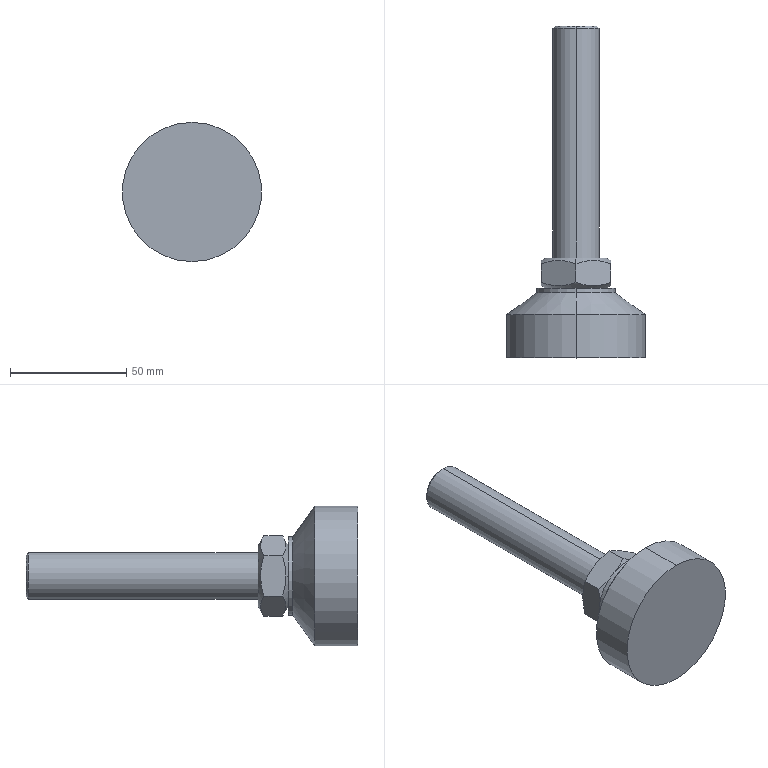Part | SolidWorks | features BaseBody 1 | 1 solid | 24 faces | box 60 x 143 x 60 mm | volume 112312 mm3 | plane 10 | cone 8 | cylinder 6 | commonest cylinder face diameters 20 x2 34 x2 60 x2
STEP:
#1=CARTESIAN_POINT('',(0.,43.,10.));
#2=VERTEX_POINT('',#1);
#3=CARTESIAN_POINT('',(0.,43.,-10.));
#4=VERTEX_POINT('',#3);
#5=CARTESIAN_POINT('',(0.,43.,0.));
#6=DIRECTION('',(0.,1.,0.));
#7=DIRECTION('',(0.,0.,1.));
#8=AXIS2_PLACEMENT_3D('',#5,#6,#7);
#9=CIRCLE('',#8,10.);
#10=EDGE_CURVE('',#2,#4,#9,.T.);
#11=ORIENTED_EDGE('',*,*,#10,.T.);
#12=CARTESIAN_POINT('',(0.,142.,-10.));
#13=VERTEX_POINT('',#12);
#14=CARTESIAN_POINT('',(0.,500.,-10.));
#15=DIRECTION('',(0.,1.,0.));
#16=VECTOR('',#15,1000.);
#17=LINE('',#14,#16);
#18=EDGE_CURVE('',#4,#13,#17,.T.);
#19=ORIENTED_EDGE('',*,*,#18,.T.);
#20=CARTESIAN_POINT('',(0.,142.,10.));
#21=VERTEX_POINT('',#20);
#22=CARTESIAN_POINT('',(0.,142.,0.));
#23=DIRECTION('',(0.,-1.,0.));
#24=DIRECTION('',(0.,0.,1.));
#25=AXIS2_PLACEMENT_3D('',#22,#23,#24);
#26=CIRCLE('',#25,10.);
#27=EDGE_CURVE('',#13,#21,#26,.T.);
#28=ORIENTED_EDGE('',*,*,#27,.T.);
#29=CARTESIAN_POINT('',(0.,500.,10.));
#30=DIRECTION('',(0.,1.,0.));
#31=VECTOR('',#30,1000.);
#32=LINE('',#29,#31);
#33=EDGE_CURVE('',#2,#21,#32,.T.);
#34=ORIENTED_EDGE('',*,*,#33,.F.);
#35=EDGE_LOOP('',(#11,#19,#28,#34));
#36=FACE_OUTER_BOUND('',#35,.T.);
#37=CARTESIAN_POINT('',(0.,500.,0.));
#38=DIRECTION('',(0.,1.,0.));
#39=DIRECTION('',(0.,0.,1.));
#40=AXIS2_PLACEMENT_3D('',#37,#38,#39);
#41=CYLINDRICAL_SURFACE('',#40,10.);
#42=ADVANCED_FACE('',(#36),#41,.T.);
#43=CARTESIAN_POINT('',(0.,143.,-9.));
#44=VERTEX_POINT('',#43);
#45=CARTESIAN_POINT('',(0.,143.,9.));
#46=VERTEX_POINT('',#45);
#47=CARTESIAN_POINT('',(0.,143.,0.));
#48=DIRECTION('',(0.,-1.,0.));
#49=DIRECTION('',(0.,0.,-1.));
#50=AXIS2_PLACEMENT_3D('',#47,#48,#49);
#51=CIRCLE('',#50,9.);
#52=EDGE_CURVE('',#44,#46,#51,.T.);
#53=ORIENTED_EDGE('',*,*,#52,.T.);
#54=CARTESIAN_POINT('',(0.,142.,10.));
#55=DIRECTION('',(0.,-0.7071,0.7071));
#56=VECTOR('',#55,1000.);
#57=LINE('',#54,#56);
#58=EDGE_CURVE('',#46,#21,#57,.T.);
#59=ORIENTED_EDGE('',*,*,#58,.T.);
#60=ORIENTED_EDGE('',*,*,#27,.F.);
#61=CARTESIAN_POINT('',(0.,142.,-10.));
#62=DIRECTION('',(0.,-0.7071,-0.7071));
#63=VECTOR('',#62,1000.);
#64=LINE('',#61,#63);
#65=EDGE_CURVE('',#44,#13,#64,.T.);
#66=ORIENTED_EDGE('',*,*,#65,.F.);
#67=EDGE_LOOP('',(#53,#59,#60,#66));
#68=FACE_OUTER_BOUND('',#67,.T.);
#69=CARTESIAN_POINT('',(0.,142.,0.));
#70=DIRECTION('',(0.,-1.,0.));
#71=DIRECTION('',(0.,0.,-1.));
#72=AXIS2_PLACEMENT_3D('',#69,#70,#71);
#73=CONICAL_SURFACE('',#72,10.,0.7854);
#74=ADVANCED_FACE('',(#68),#73,.T.);
#75=CARTESIAN_POINT('',(0.,43.,-13.1));
#76=VERTEX_POINT('',#75);
#77=CARTESIAN_POINT('',(0.,43.,13.1));
#78=VERTEX_POINT('',#77);
#79=CARTESIAN_POINT('',(0.,43.,0.));
#80=DIRECTION('',(0.,-1.,0.));
#81=DIRECTION('',(0.,0.,-1.));
#82=AXIS2_PLACEMENT_3D('',#79,#80,#81);
#83=CIRCLE('',#82,13.1);
#84=EDGE_CURVE('',#76,#78,#83,.T.);
#85=ORIENTED_EDGE('',*,*,#84,.T.);
#86=CARTESIAN_POINT('',(-0.000000029,40.563,17.321));
#87=VERTEX_POINT('',#86);
#88=CARTESIAN_POINT('',(0.,40.549,17.346));
#89=DIRECTION('',(0.,-0.5,0.866));
#90=VECTOR('',#89,1000.);
#91=LINE('',#88,#90);
#92=EDGE_CURVE('',#78,#87,#91,.T.);
#93=ORIENTED_EDGE('',*,*,#92,.T.);
#94=CARTESIAN_POINT('',(15.,40.563,8.66));
#95=VERTEX_POINT('',#94);
#96=CARTESIAN_POINT('',(-0.000000029,40.563,17.321));
#97=CARTESIAN_POINT('',(1.225,40.971,16.613));
#98=CARTESIAN_POINT('',(2.458,41.308,15.901));
#99=CARTESIAN_POINT('',(4.951,41.774,14.462));
#100=CARTESIAN_POINT('',(6.21,41.902,13.735));
#101=CARTESIAN_POINT('',(8.123,41.903,12.631));
#102=CARTESIAN_POINT('',(8.764,41.872,12.261));
#103=CARTESIAN_POINT('',(10.031,41.75,11.529));
#104=CARTESIAN_POINT('',(10.661,41.659,11.166));
#105=CARTESIAN_POINT('',(12.537,41.309,10.082));
#106=CARTESIAN_POINT('',(13.774,40.972,9.368));
#107=CARTESIAN_POINT('',(15.,40.563,8.66));
#108=B_SPLINE_CURVE_WITH_KNOTS('',3,(#96,#97,#98,#99,#100,#101,#102,#103,#104,#105,#106,#107),.UNSPECIFIED.,.F.,.F.,(4,2,2,2,2,4),(0.,0.004373,0.008746,0.01093,0.01312,0.01749),.UNSPECIFIED.);
#109=EDGE_CURVE('',#87,#95,#108,.T.);
#110=ORIENTED_EDGE('',*,*,#109,.T.);
#111=CARTESIAN_POINT('',(15.,40.563,-8.66));
#112=VERTEX_POINT('',#111);
#113=CARTESIAN_POINT('',(15.,40.563,8.66));
#114=CARTESIAN_POINT('',(15.,40.971,7.246));
#115=CARTESIAN_POINT('',(15.,41.308,5.822));
#116=CARTESIAN_POINT('',(15.,41.774,2.943));
#117=CARTESIAN_POINT('',(15.,41.902,1.489));
#118=CARTESIAN_POINT('',(15.,41.903,-0.7197));
#119=CARTESIAN_POINT('',(15.,41.872,-1.459));
#120=CARTESIAN_POINT('',(15.,41.75,-2.923));
#121=CARTESIAN_POINT('',(15.,41.659,-3.649));
#122=CARTESIAN_POINT('',(15.,41.309,-5.817));
#123=CARTESIAN_POINT('',(15.,40.972,-7.244));
#124=CARTESIAN_POINT('',(15.,40.563,-8.66));
#125=B_SPLINE_CURVE_WITH_KNOTS('',3,(#113,#114,#115,#116,#117,#118,#119,#120,#121,#122,#123,#124),.UNSPECIFIED.,.F.,.F.,(4,2,2,2,2,4),(0.,0.004373,0.008746,0.01093,0.01312,0.01749),.UNSPECIFIED.);
#126=EDGE_CURVE('',#95,#112,#125,.T.);
#127=ORIENTED_EDGE('',*,*,#126,.T.);
#128=CARTESIAN_POINT('',(-0.000000007,40.563,-17.321));
#129=VERTEX_POINT('',#128);
#130=CARTESIAN_POINT('',(15.,40.563,-8.66));
#131=CARTESIAN_POINT('',(13.775,40.971,-9.367));
#132=CARTESIAN_POINT('',(12.542,41.308,-10.079));
#133=CARTESIAN_POINT('',(10.049,41.774,-11.519));
#134=CARTESIAN_POINT('',(8.79,41.902,-12.246));
#135=CARTESIAN_POINT('',(6.877,41.903,-13.35));
#136=CARTESIAN_POINT('',(6.236,41.872,-13.72));
#137=CARTESIAN_POINT('',(4.969,41.75,-14.452));
#138=CARTESIAN_POINT('',(4.339,41.659,-14.815));
#139=CARTESIAN_POINT('',(2.463,41.309,-15.899));
#140=CARTESIAN_POINT('',(1.226,40.972,-16.613));
#141=CARTESIAN_POINT('',(-0.000000007,40.563,-17.321));
#142=B_SPLINE_CURVE_WITH_KNOTS('',3,(#130,#131,#132,#133,#134,#135,#136,#137,#138,#139,#140,#141),.UNSPECIFIED.,.F.,.F.,(4,2,2,2,2,4),(0.,0.004373,0.008746,0.01093,0.01312,0.01749),.UNSPECIFIED.);
#143=EDGE_CURVE('',#112,#129,#142,.T.);
#144=ORIENTED_EDGE('',*,*,#143,.T.);
#145=CARTESIAN_POINT('',(0.,40.549,-17.346));
#146=DIRECTION('',(0.,-0.5,-0.866));
#147=VECTOR('',#146,1000.);
#148=LINE('',#145,#147);
#149=EDGE_CURVE('',#76,#129,#148,.T.);
#150=ORIENTED_EDGE('',*,*,#149,.F.);
#151=EDGE_LOOP('',(#85,#93,#110,#127,#144,#150));
#152=FACE_OUTER_BOUND('',#151,.T.);
#153=CARTESIAN_POINT('',(0.,40.549,0.));
#154=DIRECTION('',(0.,-1.,0.));
#155=DIRECTION('',(0.,0.,-1.));
#156=AXIS2_PLACEMENT_3D('',#153,#154,#155);
#157=CONICAL_SURFACE('',#156,17.346,1.047);
#158=ADVANCED_FACE('',(#152),#157,.T.);
#159=CARTESIAN_POINT('',(-13.1,30.,0.));
#160=VERTEX_POINT('',#159);
#161=CARTESIAN_POINT('',(13.1,30.,0.));
#162=VERTEX_POINT('',#161);
#163=CARTESIAN_POINT('',(0.,30.,0.));
#164=DIRECTION('',(0.,1.,0.));
#165=DIRECTION('',(-1.,0.,0.));
#166=AXIS2_PLACEMENT_3D('',#163,#164,#165);
#167=CIRCLE('',#166,13.1);
#168=EDGE_CURVE('',#160,#162,#167,.T.);
#169=ORIENTED_EDGE('',*,*,#168,.T.);
#170=CARTESIAN_POINT('',(15.,31.097,0.));
#171=VERTEX_POINT('',#170);
#172=CARTESIAN_POINT('',(17.346,32.451,0.));
#173=DIRECTION('',(0.866,0.5,0.));
#174=VECTOR('',#173,1000.);
#175=LINE('',#172,#174);
#176=EDGE_CURVE('',#162,#171,#175,.T.);
#177=ORIENTED_EDGE('',*,*,#176,.T.);
#178=CARTESIAN_POINT('',(15.,32.437,8.66));
#179=VERTEX_POINT('',#178);
#180=CARTESIAN_POINT('',(15.,31.097,0.));
#181=CARTESIAN_POINT('',(15.,31.097,0.735));
#182=CARTESIAN_POINT('',(15.,31.129,1.473));
#183=CARTESIAN_POINT('',(15.,31.251,2.934));
#184=CARTESIAN_POINT('',(15.,31.342,3.659));
#185=CARTESIAN_POINT('',(15.,31.692,5.822));
#186=CARTESIAN_POINT('',(15.,32.029,7.247));
#187=CARTESIAN_POINT('',(15.,32.437,8.66));
#188=B_SPLINE_CURVE_WITH_KNOTS('',3,(#180,#181,#182,#183,#184,#185,#186,#187),.UNSPECIFIED.,.F.,.F.,(4,2,2,4),(0.008763,0.01095,0.01313,0.01749),.UNSPECIFIED.);
#189=EDGE_CURVE('',#171,#179,#188,.T.);
#190=ORIENTED_EDGE('',*,*,#189,.T.);
#191=CARTESIAN_POINT('',(0.,32.437,17.321));
#192=VERTEX_POINT('',#191);
#193=CARTESIAN_POINT('',(15.,32.437,8.66));
#194=CARTESIAN_POINT('',(13.775,32.029,9.367));
#195=CARTESIAN_POINT('',(12.542,31.692,10.079));
#196=CARTESIAN_POINT('',(10.049,31.226,11.519));
#197=CARTESIAN_POINT('',(8.79,31.098,12.246));
#198=CARTESIAN_POINT('',(6.877,31.097,13.35));
#199=CARTESIAN_POINT('',(6.236,31.128,13.72));
#200=CARTESIAN_POINT('',(4.969,31.25,14.452));
#201=CARTESIAN_POINT('',(4.339,31.341,14.815));
#202=CARTESIAN_POINT('',(2.463,31.691,15.899));
#203=CARTESIAN_POINT('',(1.226,32.028,16.613));
#204=CARTESIAN_POINT('',(0.,32.437,17.321));
#205=B_SPLINE_CURVE_WITH_KNOTS('',3,(#193,#194,#195,#196,#197,#198,#199,#200,#201,#202,#203,#204),.UNSPECIFIED.,.F.,.F.,(4,2,2,2,2,4),(0.,0.004373,0.008746,0.01093,0.01312,0.01749),.UNSPECIFIED.);
#206=EDGE_CURVE('',#179,#192,#205,.T.);
#207=ORIENTED_EDGE('',*,*,#206,.T.);
#208=CARTESIAN_POINT('',(-15.,32.437,8.66));
#209=VERTEX_POINT('',#208);
#210=CARTESIAN_POINT('',(0.,32.437,17.321));
#211=CARTESIAN_POINT('',(-1.225,32.029,16.613));
#212=CARTESIAN_POINT('',(-2.458,31.692,15.901));
#213=CARTESIAN_POINT('',(-4.951,31.226,14.462));
#214=CARTESIAN_POINT('',(-6.21,31.098,13.735));
#215=CARTESIAN_POINT('',(-8.123,31.097,12.631));
#216=CARTESIAN_POINT('',(-8.764,31.128,12.261));
#217=CARTESIAN_POINT('',(-10.031,31.25,11.529));
#218=CARTESIAN_POINT('',(-10.661,31.341,11.166));
#219=CARTESIAN_POINT('',(-12.537,31.691,10.082));
#220=CARTESIAN_POINT('',(-13.774,32.028,9.368));
#221=CARTESIAN_POINT('',(-15.,32.437,8.66));
#222=B_SPLINE_CURVE_WITH_KNOTS('',3,(#210,#211,#212,#213,#214,#215,#216,#217,#218,#219,#220,#221),.UNSPECIFIED.,.F.,.F.,(4,2,2,2,2,4),(0.,0.004373,0.008746,0.01093,0.01312,0.01749),.UNSPECIFIED.);
#223=EDGE_CURVE('',#192,#209,#222,.T.);
#224=ORIENTED_EDGE('',*,*,#223,.T.);
#225=CARTESIAN_POINT('',(-15.,31.097,0.));
#226=VERTEX_POINT('',#225);
#227=CARTESIAN_POINT('',(-15.,32.437,8.66));
#228=CARTESIAN_POINT('',(-15.,32.028,7.244));
#229=CARTESIAN_POINT('',(-15.,31.691,5.816));
#230=CARTESIAN_POINT('',(-15.,31.225,2.933));
#231=CARTESIAN_POINT('',(-15.,31.097,1.475));
#232=CARTESIAN_POINT('',(-15.,31.097,0.));
#233=B_SPLINE_CURVE_WITH_KNOTS('',3,(#227,#228,#229,#230,#231,#232),.UNSPECIFIED.,.F.,.F.,(4,2,4),(0.,0.004381,0.008763),.UNSPECIFIED.);
#234=EDGE_CURVE('',#209,#226,#233,.T.);
#235=ORIENTED_EDGE('',*,*,#234,.T.);
#236=CARTESIAN_POINT('',(-17.346,32.451,0.));
#237=DIRECTION('',(-0.866,0.5,0.));
#238=VECTOR('',#237,1000.);
#239=LINE('',#236,#238);
#240=EDGE_CURVE('',#160,#226,#239,.T.);
#241=ORIENTED_EDGE('',*,*,#240,.F.);
#242=EDGE_LOOP('',(#169,#177,#190,#207,#224,#235,#241));
#243=FACE_OUTER_BOUND('',#242,.T.);
#244=CARTESIAN_POINT('',(0.,32.451,0.));
#245=DIRECTION('',(0.,1.,0.));
#246=DIRECTION('',(-1.,0.,0.));
#247=AXIS2_PLACEMENT_3D('',#244,#245,#246);
#248=CONICAL_SURFACE('',#247,17.346,1.047);
#249=ADVANCED_FACE('',(#243),#248,.T.);
#250=CARTESIAN_POINT('',(0.,28.,17.));
#251=VERTEX_POINT('',#250);
#252=CARTESIAN_POINT('',(0.,28.,-17.));
#253=VERTEX_POINT('',#252);
#254=CARTESIAN_POINT('',(0.,28.,0.));
#255=DIRECTION('',(0.,1.,0.));
#256=DIRECTION('',(0.,0.,1.));
#257=AXIS2_PLACEMENT_3D('',#254,#255,#256);
#258=CIRCLE('',#257,17.);
#259=EDGE_CURVE('',#251,#253,#258,.T.);
#260=ORIENTED_EDGE('',*,*,#259,.T.);
#261=CARTESIAN_POINT('',(0.,30.,-17.));
#262=VERTEX_POINT('',#261);
#263=CARTESIAN_POINT('',(0.,500.,-17.));
#264=DIRECTION('',(0.,1.,0.));
#265=VECTOR('',#264,1000.);
#266=LINE('',#263,#265);
#267=EDGE_CURVE('',#253,#262,#266,.T.);
#268=ORIENTED_EDGE('',*,*,#267,.T.);
#269=CARTESIAN_POINT('',(0.,30.,17.));
#270=VERTEX_POINT('',#269);
#271=CARTESIAN_POINT('',(0.,30.,0.));
#272=DIRECTION('',(0.,-1.,0.));
#273=DIRECTION('',(0.,0.,1.));
#274=AXIS2_PLACEMENT_3D('',#271,#272,#273);
#275=CIRCLE('',#274,17.);
#276=EDGE_CURVE('',#262,#270,#275,.T.);
#277=ORIENTED_EDGE('',*,*,#276,.T.);
#278=CARTESIAN_POINT('',(0.,500.,17.));
#279=DIRECTION('',(0.,1.,0.));
#280=VECTOR('',#279,1000.);
#281=LINE('',#278,#280);
#282=EDGE_CURVE('',#251,#270,#281,.T.);
#283=ORIENTED_EDGE('',*,*,#282,.F.);
#284=EDGE_LOOP('',(#260,#268,#277,#283));
#285=FACE_OUTER_BOUND('',#284,.T.);
#286=CARTESIAN_POINT('',(0.,500.,0.));
#287=DIRECTION('',(0.,1.,0.));
#288=DIRECTION('',(0.,0.,1.));
#289=AXIS2_PLACEMENT_3D('',#286,#287,#288);
#290=CYLINDRICAL_SURFACE('',#289,17.);
#291=ADVANCED_FACE('',(#285),#290,.T.);
#292=ORIENTED_EDGE('',*,*,#259,.F.);
#293=CARTESIAN_POINT('',(0.,18.667,30.));
#294=VERTEX_POINT('',#293);
#295=CARTESIAN_POINT('',(0.,18.667,30.));
#296=DIRECTION('',(0.,-0.5832,0.8123));
#297=VECTOR('',#296,1000.);
#298=LINE('',#295,#297);
#299=EDGE_CURVE('',#251,#294,#298,.T.);
#300=ORIENTED_EDGE('',*,*,#299,.T.);
#301=CARTESIAN_POINT('',(0.,18.667,-30.));
#302=VERTEX_POINT('',#301);
#303=CARTESIAN_POINT('',(0.,18.667,0.));
#304=DIRECTION('',(0.,1.,0.));
#305=DIRECTION('',(0.,0.,-1.));
#306=AXIS2_PLACEMENT_3D('',#303,#304,#305);
#307=CIRCLE('',#306,30.);
#308=EDGE_CURVE('',#294,#302,#307,.T.);
#309=ORIENTED_EDGE('',*,*,#308,.T.);
#310=CARTESIAN_POINT('',(0.,18.667,-30.));
#311=DIRECTION('',(0.,-0.5832,-0.8123));
#312=VECTOR('',#311,1000.);
#313=LINE('',#310,#312);
#314=EDGE_CURVE('',#253,#302,#313,.T.);
#315=ORIENTED_EDGE('',*,*,#314,.F.);
#316=EDGE_LOOP('',(#292,#300,#309,#315));
#317=FACE_OUTER_BOUND('',#316,.T.);
#318=CARTESIAN_POINT('',(0.,18.667,0.));
#319=DIRECTION('',(0.,-1.,0.));
#320=DIRECTION('',(0.,0.,-1.));
#321=AXIS2_PLACEMENT_3D('',#318,#319,#320);
#322=CONICAL_SURFACE('',#321,30.,0.9481);
#323=ADVANCED_FACE('',(#317),#322,.T.);
#324=CARTESIAN_POINT('',(0.,0.,30.));
#325=VERTEX_POINT('',#324);
#326=CARTESIAN_POINT('',(0.,0.,-30.));
#327=VERTEX_POINT('',#326);
#328=CARTESIAN_POINT('',(0.,0.,0.));
#329=DIRECTION('',(0.,1.,0.));
#330=DIRECTION('',(0.,0.,1.));
#331=AXIS2_PLACEMENT_3D('',#328,#329,#330);
#332=CIRCLE('',#331,30.);
#333=EDGE_CURVE('',#325,#327,#332,.T.);
#334=ORIENTED_EDGE('',*,*,#333,.T.);
#335=CARTESIAN_POINT('',(0.,500.,-30.));
#336=DIRECTION('',(0.,1.,0.));
#337=VECTOR('',#336,1000.);
#338=LINE('',#335,#337);
#339=EDGE_CURVE('',#327,#302,#338,.T.);
#340=ORIENTED_EDGE('',*,*,#339,.T.);
#341=ORIENTED_EDGE('',*,*,#308,.F.);
#342=CARTESIAN_POINT('',(0.,500.,30.));
#343=DIRECTION('',(0.,1.,0.));
#344=VECTOR('',#343,1000.);
#345=LINE('',#342,#344);
#346=EDGE_CURVE('',#325,#294,#345,.T.);
#347=ORIENTED_EDGE('',*,*,#346,.F.);
#348=EDGE_LOOP('',(#334,#340,#341,#347));
#349=FACE_OUTER_BOUND('',#348,.T.);
#350=CARTESIAN_POINT('',(0.,500.,0.));
#351=DIRECTION('',(0.,1.,0.));
#352=DIRECTION('',(0.,0.,1.));
#353=AXIS2_PLACEMENT_3D('',#350,#351,#352);
#354=CYLINDRICAL_SURFACE('',#353,30.);
#355=ADVANCED_FACE('',(#349),#354,.T.);
#356=ORIENTED_EDGE('',*,*,#18,.F.);
#357=CARTESIAN_POINT('',(0.,43.,0.));
#358=DIRECTION('',(0.,1.,0.));
#359=DIRECTION('',(0.,0.,1.));
#360=AXIS2_PLACEMENT_3D('',#357,#358,#359);
#361=CIRCLE('',#360,10.);
#362=EDGE_CURVE('',#4,#2,#361,.T.);
#363=ORIENTED_EDGE('',*,*,#362,.T.);
#364=ORIENTED_EDGE('',*,*,#33,.T.);
#365=CARTESIAN_POINT('',(0.,142.,0.));
#366=DIRECTION('',(0.,-1.,0.));
#367=DIRECTION('',(0.,0.,1.));
#368=AXIS2_PLACEMENT_3D('',#365,#366,#367);
#369=CIRCLE('',#368,10.);
#370=EDGE_CURVE('',#21,#13,#369,.T.);
#371=ORIENTED_EDGE('',*,*,#370,.T.);
#372=EDGE_LOOP('',(#356,#363,#364,#371));
#373=FACE_OUTER_BOUND('',#372,.T.);
#374=CARTESIAN_POINT('',(0.,500.,0.));
#375=DIRECTION('',(0.,1.,0.));
#376=DIRECTION('',(0.,0.,1.));
#377=AXIS2_PLACEMENT_3D('',#374,#375,#376);
#378=CYLINDRICAL_SURFACE('',#377,10.);
#379=ADVANCED_FACE('',(#373),#378,.T.);
#380=ORIENTED_EDGE('',*,*,#84,.F.);
#381=CARTESIAN_POINT('',(0.,43.,0.));
#382=DIRECTION('',(0.,-1.,0.));
#383=DIRECTION('',(0.,0.,-1.));
#384=AXIS2_PLACEMENT_3D('',#381,#382,#383);
#385=CIRCLE('',#384,13.1);
#386=EDGE_CURVE('',#78,#76,#385,.T.);
#387=ORIENTED_EDGE('',*,*,#386,.F.);
#388=EDGE_LOOP('',(#380,#387));
#389=FACE_OUTER_BOUND('',#388,.T.);
#390=ORIENTED_EDGE('',*,*,#10,.F.);
#391=ORIENTED_EDGE('',*,*,#362,.F.);
#392=EDGE_LOOP('',(#390,#391));
#393=FACE_BOUND('',#392,.T.);
#394=CARTESIAN_POINT('',(0.,43.,13.1));
#395=DIRECTION('',(0.,-1.,0.));
#396=DIRECTION('',(0.,0.,-1.));
#397=AXIS2_PLACEMENT_3D('',#394,#395,#396);
#398=PLANE('',#397);
#399=ADVANCED_FACE('',(#389,#393),#398,.F.);
#400=ORIENTED_EDGE('',*,*,#58,.F.);
#401=CARTESIAN_POINT('',(0.,143.,0.));
#402=DIRECTION('',(0.,-1.,0.));
#403=DIRECTION('',(0.,0.,-1.));
#404=AXIS2_PLACEMENT_3D('',#401,#402,#403);
#405=CIRCLE('',#404,9.);
#406=EDGE_CURVE('',#46,#44,#405,.T.);
#407=ORIENTED_EDGE('',*,*,#406,.T.);
#408=ORIENTED_EDGE('',*,*,#65,.T.);
#409=ORIENTED_EDGE('',*,*,#370,.F.);
#410=EDGE_LOOP('',(#400,#407,#408,#409));
#411=FACE_OUTER_BOUND('',#410,.T.);
#412=CARTESIAN_POINT('',(0.,142.,0.));
#413=DIRECTION('',(0.,-1.,0.));
#414=DIRECTION('',(0.,0.,-1.));
#415=AXIS2_PLACEMENT_3D('',#412,#413,#414);
#416=CONICAL_SURFACE('',#415,10.,0.7854);
#417=ADVANCED_FACE('',(#411),#416,.T.);
#418=ORIENTED_EDGE('',*,*,#92,.F.);
#419=ORIENTED_EDGE('',*,*,#386,.T.);
#420=ORIENTED_EDGE('',*,*,#149,.T.);
#421=CARTESIAN_POINT('',(-15.,40.563,-8.66));
#422=VERTEX_POINT('',#421);
#423=CARTESIAN_POINT('',(-0.000000007,40.563,-17.321));
#424=CARTESIAN_POINT('',(-1.225,40.971,-16.613));
#425=CARTESIAN_POINT('',(-2.458,41.308,-15.901));
#426=CARTESIAN_POINT('',(-4.951,41.774,-14.462));
#427=CARTESIAN_POINT('',(-6.21,41.902,-13.735));
#428=CARTESIAN_POINT('',(-8.123,41.903,-12.631));
#429=CARTESIAN_POINT('',(-8.764,41.872,-12.261));
#430=CARTESIAN_POINT('',(-10.031,41.75,-11.529));
#431=CARTESIAN_POINT('',(-10.661,41.659,-11.166));
#432=CARTESIAN_POINT('',(-12.537,41.309,-10.082));
#433=CARTESIAN_POINT('',(-13.774,40.972,-9.368));
#434=CARTESIAN_POINT('',(-15.,40.563,-8.66));
#435=B_SPLINE_CURVE_WITH_KNOTS('',3,(#423,#424,#425,#426,#427,#428,#429,#430,#431,#432,#433,#434),.UNSPECIFIED.,.F.,.F.,(4,2,2,2,2,4),(0.,0.004373,0.008746,0.01093,0.01312,0.01749),.UNSPECIFIED.);
#436=EDGE_CURVE('',#129,#422,#435,.T.);
#437=ORIENTED_EDGE('',*,*,#436,.T.);
#438=CARTESIAN_POINT('',(-15.,40.563,8.66));
#439=VERTEX_POINT('',#438);
#440=CARTESIAN_POINT('',(-15.,40.563,-8.66));
#441=CARTESIAN_POINT('',(-15.,40.971,-7.246));
#442=CARTESIAN_POINT('',(-15.,41.308,-5.822));
#443=CARTESIAN_POINT('',(-15.,41.774,-2.943));
#444=CARTESIAN_POINT('',(-15.,41.902,-1.489));
#445=CARTESIAN_POINT('',(-15.,41.903,0.7197));
#446=CARTESIAN_POINT('',(-15.,41.872,1.459));
#447=CARTESIAN_POINT('',(-15.,41.75,2.923));
#448=CARTESIAN_POINT('',(-15.,41.659,3.649));
#449=CARTESIAN_POINT('',(-15.,41.309,5.817));
#450=CARTESIAN_POINT('',(-15.,40.972,7.244));
#451=CARTESIAN_POINT('',(-15.,40.563,8.66));
#452=B_SPLINE_CURVE_WITH_KNOTS('',3,(#440,#441,#442,#443,#444,#445,#446,#447,#448,#449,#450,#451),.UNSPECIFIED.,.F.,.F.,(4,2,2,2,2,4),(0.,0.004373,0.008746,0.01093,0.01312,0.01749),.UNSPECIFIED.);
#453=EDGE_CURVE('',#422,#439,#452,.T.);
#454=ORIENTED_EDGE('',*,*,#453,.T.);
#455=CARTESIAN_POINT('',(-15.,40.563,8.66));
#456=CARTESIAN_POINT('',(-13.775,40.971,9.367));
#457=CARTESIAN_POINT('',(-12.542,41.308,10.079));
#458=CARTESIAN_POINT('',(-10.049,41.774,11.519));
#459=CARTESIAN_POINT('',(-8.79,41.902,12.246));
#460=CARTESIAN_POINT('',(-6.877,41.903,13.35));
#461=CARTESIAN_POINT('',(-6.236,41.872,13.72));
#462=CARTESIAN_POINT('',(-4.969,41.75,14.452));
#463=CARTESIAN_POINT('',(-4.339,41.659,14.815));
#464=CARTESIAN_POINT('',(-2.463,41.309,15.899));
#465=CARTESIAN_POINT('',(-1.226,40.972,16.613));
#466=CARTESIAN_POINT('',(-0.000000029,40.563,17.321));
#467=B_SPLINE_CURVE_WITH_KNOTS('',3,(#455,#456,#457,#458,#459,#460,#461,#462,#463,#464,#465,#466),.UNSPECIFIED.,.F.,.F.,(4,2,2,2,2,4),(0.,0.004373,0.008746,0.01093,0.01312,0.01749),.UNSPECIFIED.);
#468=EDGE_CURVE('',#439,#87,#467,.T.);
#469=ORIENTED_EDGE('',*,*,#468,.T.);
#470=EDGE_LOOP('',(#418,#419,#420,#437,#454,#469));
#471=FACE_OUTER_BOUND('',#470,.T.);
#472=CARTESIAN_POINT('',(0.,40.549,0.));
#473=DIRECTION('',(0.,-1.,0.));
#474=DIRECTION('',(0.,0.,-1.));
#475=AXIS2_PLACEMENT_3D('',#472,#473,#474);
#476=CONICAL_SURFACE('',#475,17.346,1.047);
#477=ADVANCED_FACE('',(#471),#476,.T.);
#478=ORIENTED_EDGE('',*,*,#52,.F.);
#479=ORIENTED_EDGE('',*,*,#406,.F.);
#480=EDGE_LOOP('',(#478,#479));
#481=FACE_OUTER_BOUND('',#480,.T.);
#482=CARTESIAN_POINT('',(0.,143.,9.));
#483=DIRECTION('',(0.,-1.,0.));
#484=DIRECTION('',(0.,0.,-1.));
#485=AXIS2_PLACEMENT_3D('',#482,#483,#484);
#486=PLANE('',#485);
#487=ADVANCED_FACE('',(#481),#486,.F.);
#488=ORIENTED_EDGE('',*,*,#143,.F.);
#489=CARTESIAN_POINT('',(15.,32.437,-8.66));
#490=VERTEX_POINT('',#489);
#491=CARTESIAN_POINT('',(15.,43.,-8.66));
#492=DIRECTION('',(0.,1.,0.));
#493=VECTOR('',#492,1000.);
#494=LINE('',#491,#493);
#495=EDGE_CURVE('',#490,#112,#494,.T.);
#496=ORIENTED_EDGE('',*,*,#495,.F.);
#497=CARTESIAN_POINT('',(0.,32.437,-17.321));
#498=VERTEX_POINT('',#497);
#499=CARTESIAN_POINT('',(0.,32.437,-17.321));
#500=CARTESIAN_POINT('',(1.225,32.029,-16.613));
#501=CARTESIAN_POINT('',(2.458,31.692,-15.901));
#502=CARTESIAN_POINT('',(4.951,31.226,-14.462));
#503=CARTESIAN_POINT('',(6.21,31.098,-13.735));
#504=CARTESIAN_POINT('',(8.123,31.097,-12.631));
#505=CARTESIAN_POINT('',(8.764,31.128,-12.261));
#506=CARTESIAN_POINT('',(10.031,31.25,-11.529));
#507=CARTESIAN_POINT('',(10.661,31.341,-11.166));
#508=CARTESIAN_POINT('',(12.537,31.691,-10.082));
#509=CARTESIAN_POINT('',(13.774,32.028,-9.368));
#510=CARTESIAN_POINT('',(15.,32.437,-8.66));
#511=B_SPLINE_CURVE_WITH_KNOTS('',3,(#499,#500,#501,#502,#503,#504,#505,#506,#507,#508,#509,#510),.UNSPECIFIED.,.F.,.F.,(4,2,2,2,2,4),(0.,0.004373,0.008746,0.01093,0.01312,0.01749),.UNSPECIFIED.);
#512=EDGE_CURVE('',#498,#490,#511,.T.);
#513=ORIENTED_EDGE('',*,*,#512,.F.);
#514=CARTESIAN_POINT('',(0.,43.,-17.321));
#515=DIRECTION('',(0.,-1.,0.));
#516=VECTOR('',#515,1000.);
#517=LINE('',#514,#516);
#518=EDGE_CURVE('',#129,#498,#517,.T.);
#519=ORIENTED_EDGE('',*,*,#518,.F.);
#520=EDGE_LOOP('',(#488,#496,#513,#519));
#521=FACE_OUTER_BOUND('',#520,.T.);
#522=CARTESIAN_POINT('',(15.,43.,-8.66));
#523=DIRECTION('',(-0.5,0.,0.866));
#524=DIRECTION('',(0.866,0.,0.5));
#525=AXIS2_PLACEMENT_3D('',#522,#523,#524);
#526=PLANE('',#525);
#527=ADVANCED_FACE('',(#521),#526,.F.);
#528=ORIENTED_EDGE('',*,*,#126,.F.);
#529=CARTESIAN_POINT('',(15.,43.,8.66));
#530=DIRECTION('',(0.,1.,0.));
#531=VECTOR('',#530,1000.);
#532=LINE('',#529,#531);
#533=EDGE_CURVE('',#179,#95,#532,.T.);
#534=ORIENTED_EDGE('',*,*,#533,.F.);
#535=ORIENTED_EDGE('',*,*,#189,.F.);
#536=CARTESIAN_POINT('',(15.,32.437,-8.66));
#537=CARTESIAN_POINT('',(15.,32.028,-7.244));
#538=CARTESIAN_POINT('',(15.,31.691,-5.816));
#539=CARTESIAN_POINT('',(15.,31.225,-2.933));
#540=CARTESIAN_POINT('',(15.,31.097,-1.475));
#541=CARTESIAN_POINT('',(15.,31.097,0.));
#542=B_SPLINE_CURVE_WITH_KNOTS('',3,(#536,#537,#538,#539,#540,#541),.UNSPECIFIED.,.F.,.F.,(4,2,4),(0.,0.004381,0.008763),.UNSPECIFIED.);
#543=EDGE_CURVE('',#490,#171,#542,.T.);
#544=ORIENTED_EDGE('',*,*,#543,.F.);
#545=ORIENTED_EDGE('',*,*,#495,.T.);
#546=EDGE_LOOP('',(#528,#534,#535,#544,#545));
#547=FACE_OUTER_BOUND('',#546,.T.);
#548=CARTESIAN_POINT('',(15.,43.,8.66));
#549=DIRECTION('',(-1.,0.,0.));
#550=DIRECTION('',(0.,0.,1.));
#551=AXIS2_PLACEMENT_3D('',#548,#549,#550);
#552=PLANE('',#551);
#553=ADVANCED_FACE('',(#547),#552,.F.);
#554=ORIENTED_EDGE('',*,*,#109,.F.);
#555=CARTESIAN_POINT('',(0.,43.,17.321));
#556=DIRECTION('',(0.,1.,0.));
#557=VECTOR('',#556,1000.);
#558=LINE('',#555,#557);
#559=EDGE_CURVE('',#192,#87,#558,.T.);
#560=ORIENTED_EDGE('',*,*,#559,.F.);
#561=ORIENTED_EDGE('',*,*,#206,.F.);
#562=ORIENTED_EDGE('',*,*,#533,.T.);
#563=EDGE_LOOP('',(#554,#560,#561,#562));
#564=FACE_OUTER_BOUND('',#563,.T.);
#565=CARTESIAN_POINT('',(0.,43.,17.321));
#566=DIRECTION('',(-0.5,0.,-0.866));
#567=DIRECTION('',(-0.866,0.,0.5));
#568=AXIS2_PLACEMENT_3D('',#565,#566,#567);
#569=PLANE('',#568);
#570=ADVANCED_FACE('',(#564),#569,.F.);
#571=ORIENTED_EDGE('',*,*,#468,.F.);
#572=CARTESIAN_POINT('',(-15.,43.,8.66));
#573=DIRECTION('',(0.,1.,0.));
#574=VECTOR('',#573,1000.);
#575=LINE('',#572,#574);
#576=EDGE_CURVE('',#209,#439,#575,.T.);
#577=ORIENTED_EDGE('',*,*,#576,.F.);
#578=ORIENTED_EDGE('',*,*,#223,.F.);
#579=ORIENTED_EDGE('',*,*,#559,.T.);
#580=EDGE_LOOP('',(#571,#577,#578,#579));
#581=FACE_OUTER_BOUND('',#580,.T.);
#582=CARTESIAN_POINT('',(-15.,43.,8.66));
#583=DIRECTION('',(0.5,0.,-0.866));
#584=DIRECTION('',(-0.866,0.,-0.5));
#585=AXIS2_PLACEMENT_3D('',#582,#583,#584);
#586=PLANE('',#585);
#587=ADVANCED_FACE('',(#581),#586,.F.);
#588=ORIENTED_EDGE('',*,*,#453,.F.);
#589=CARTESIAN_POINT('',(-15.,32.437,-8.66));
#590=VERTEX_POINT('',#589);
#591=CARTESIAN_POINT('',(-15.,43.,-8.66));
#592=DIRECTION('',(0.,1.,0.));
#593=VECTOR('',#592,1000.);
#594=LINE('',#591,#593);
#595=EDGE_CURVE('',#590,#422,#594,.T.);
#596=ORIENTED_EDGE('',*,*,#595,.F.);
#597=CARTESIAN_POINT('',(-15.,31.097,0.));
#598=CARTESIAN_POINT('',(-15.,31.097,-0.735));
#599=CARTESIAN_POINT('',(-15.,31.129,-1.473));
#600=CARTESIAN_POINT('',(-15.,31.251,-2.934));
#601=CARTESIAN_POINT('',(-15.,31.342,-3.659));
#602=CARTESIAN_POINT('',(-15.,31.692,-5.822));
#603=CARTESIAN_POINT('',(-15.,32.029,-7.247));
#604=CARTESIAN_POINT('',(-15.,32.437,-8.66));
#605=B_SPLINE_CURVE_WITH_KNOTS('',3,(#597,#598,#599,#600,#601,#602,#603,#604),.UNSPECIFIED.,.F.,.F.,(4,2,2,4),(0.008763,0.01095,0.01313,0.01749),.UNSPECIFIED.);
#606=EDGE_CURVE('',#226,#590,#605,.T.);
#607=ORIENTED_EDGE('',*,*,#606,.F.);
#608=ORIENTED_EDGE('',*,*,#234,.F.);
#609=ORIENTED_EDGE('',*,*,#576,.T.);
#610=EDGE_LOOP('',(#588,#596,#607,#608,#609));
#611=FACE_OUTER_BOUND('',#610,.T.);
#612=CARTESIAN_POINT('',(-15.,43.,-8.66));
#613=DIRECTION('',(1.,0.,0.));
#614=DIRECTION('',(0.,0.,-1.));
#615=AXIS2_PLACEMENT_3D('',#612,#613,#614);
#616=PLANE('',#615);
#617=ADVANCED_FACE('',(#611),#616,.F.);
#618=ORIENTED_EDGE('',*,*,#436,.F.);
#619=ORIENTED_EDGE('',*,*,#518,.T.);
#620=CARTESIAN_POINT('',(-15.,32.437,-8.66));
#621=CARTESIAN_POINT('',(-13.775,32.029,-9.367));
#622=CARTESIAN_POINT('',(-12.542,31.692,-10.079));
#623=CARTESIAN_POINT('',(-10.049,31.226,-11.519));
#624=CARTESIAN_POINT('',(-8.79,31.098,-12.246));
#625=CARTESIAN_POINT('',(-6.877,31.097,-13.35));
#626=CARTESIAN_POINT('',(-6.236,31.128,-13.72));
#627=CARTESIAN_POINT('',(-4.969,31.25,-14.452));
#628=CARTESIAN_POINT('',(-4.339,31.341,-14.815));
#629=CARTESIAN_POINT('',(-2.463,31.691,-15.899));
#630=CARTESIAN_POINT('',(-1.226,32.028,-16.613));
#631=CARTESIAN_POINT('',(0.,32.437,-17.321));
#632=B_SPLINE_CURVE_WITH_KNOTS('',3,(#620,#621,#622,#623,#624,#625,#626,#627,#628,#629,#630,#631),.UNSPECIFIED.,.F.,.F.,(4,2,2,2,2,4),(0.,0.004373,0.008746,0.01093,0.01312,0.01749),.UNSPECIFIED.);
#633=EDGE_CURVE('',#590,#498,#632,.T.);
#634=ORIENTED_EDGE('',*,*,#633,.F.);
#635=ORIENTED_EDGE('',*,*,#595,.T.);
#636=EDGE_LOOP('',(#618,#619,#634,#635));
#637=FACE_OUTER_BOUND('',#636,.T.);
#638=CARTESIAN_POINT('',(0.,43.,-17.321));
#639=DIRECTION('',(0.5,0.,0.866));
#640=DIRECTION('',(0.866,0.,-0.5));
#641=AXIS2_PLACEMENT_3D('',#638,#639,#640);
#642=PLANE('',#641);
#643=ADVANCED_FACE('',(#637),#642,.F.);
#644=ORIENTED_EDGE('',*,*,#176,.F.);
#645=CARTESIAN_POINT('',(0.,30.,0.));
#646=DIRECTION('',(0.,1.,0.));
#647=DIRECTION('',(-1.,0.,0.));
#648=AXIS2_PLACEMENT_3D('',#645,#646,#647);
#649=CIRCLE('',#648,13.1);
#650=EDGE_CURVE('',#162,#160,#649,.T.);
#651=ORIENTED_EDGE('',*,*,#650,.T.);
#652=ORIENTED_EDGE('',*,*,#240,.T.);
#653=ORIENTED_EDGE('',*,*,#606,.T.);
#654=ORIENTED_EDGE('',*,*,#633,.T.);
#655=ORIENTED_EDGE('',*,*,#512,.T.);
#656=ORIENTED_EDGE('',*,*,#543,.T.);
#657=EDGE_LOOP('',(#644,#651,#652,#653,#654,#655,#656));
#658=FACE_OUTER_BOUND('',#657,.T.);
#659=CARTESIAN_POINT('',(0.,32.451,0.));
#660=DIRECTION('',(0.,1.,0.));
#661=DIRECTION('',(-1.,0.,0.));
#662=AXIS2_PLACEMENT_3D('',#659,#660,#661);
#663=CONICAL_SURFACE('',#662,17.346,1.047);
#664=ADVANCED_FACE('',(#658),#663,.T.);
#665=CARTESIAN_POINT('',(0.,30.,0.));
#666=DIRECTION('',(0.,-1.,0.));
#667=DIRECTION('',(0.,0.,1.));
#668=AXIS2_PLACEMENT_3D('',#665,#666,#667);
#669=CIRCLE('',#668,17.);
#670=EDGE_CURVE('',#270,#262,#669,.T.);
#671=ORIENTED_EDGE('',*,*,#670,.F.);
#672=ORIENTED_EDGE('',*,*,#276,.F.);
#673=EDGE_LOOP('',(#671,#672));
#674=FACE_OUTER_BOUND('',#673,.T.);
#675=ORIENTED_EDGE('',*,*,#168,.F.);
#676=ORIENTED_EDGE('',*,*,#650,.F.);
#677=EDGE_LOOP('',(#675,#676));
#678=FACE_BOUND('',#677,.T.);
#679=CARTESIAN_POINT('',(0.,30.,17.));
#680=DIRECTION('',(0.,-1.,0.));
#681=DIRECTION('',(0.,0.,-1.));
#682=AXIS2_PLACEMENT_3D('',#679,#680,#681);
#683=PLANE('',#682);
#684=ADVANCED_FACE('',(#674,#678),#683,.F.);
#685=ORIENTED_EDGE('',*,*,#267,.F.);
#686=CARTESIAN_POINT('',(0.,28.,0.));
#687=DIRECTION('',(0.,1.,0.));
#688=DIRECTION('',(0.,0.,1.));
#689=AXIS2_PLACEMENT_3D('',#686,#687,#688);
#690=CIRCLE('',#689,17.);
#691=EDGE_CURVE('',#253,#251,#690,.T.);
#692=ORIENTED_EDGE('',*,*,#691,.T.);
#693=ORIENTED_EDGE('',*,*,#282,.T.);
#694=ORIENTED_EDGE('',*,*,#670,.T.);
#695=EDGE_LOOP('',(#685,#692,#693,#694));
#696=FACE_OUTER_BOUND('',#695,.T.);
#697=CARTESIAN_POINT('',(0.,500.,0.));
#698=DIRECTION('',(0.,1.,0.));
#699=DIRECTION('',(0.,0.,1.));
#700=AXIS2_PLACEMENT_3D('',#697,#698,#699);
#701=CYLINDRICAL_SURFACE('',#700,17.);
#702=ADVANCED_FACE('',(#696),#701,.T.);
#703=ORIENTED_EDGE('',*,*,#299,.F.);
#704=ORIENTED_EDGE('',*,*,#691,.F.);
#705=ORIENTED_EDGE('',*,*,#314,.T.);
#706=CARTESIAN_POINT('',(0.,18.667,0.));
#707=DIRECTION('',(0.,1.,0.));
#708=DIRECTION('',(0.,0.,-1.));
#709=AXIS2_PLACEMENT_3D('',#706,#707,#708);
#710=CIRCLE('',#709,30.);
#711=EDGE_CURVE('',#302,#294,#710,.T.);
#712=ORIENTED_EDGE('',*,*,#711,.T.);
#713=EDGE_LOOP('',(#703,#704,#705,#712));
#714=FACE_OUTER_BOUND('',#713,.T.);
#715=CARTESIAN_POINT('',(0.,18.667,0.));
#716=DIRECTION('',(0.,-1.,0.));
#717=DIRECTION('',(0.,0.,-1.));
#718=AXIS2_PLACEMENT_3D('',#715,#716,#717);
#719=CONICAL_SURFACE('',#718,30.,0.9481);
#720=ADVANCED_FACE('',(#714),#719,.T.);
#721=ORIENTED_EDGE('',*,*,#339,.F.);
#722=CARTESIAN_POINT('',(0.,0.,0.));
#723=DIRECTION('',(0.,1.,0.));
#724=DIRECTION('',(0.,0.,1.));
#725=AXIS2_PLACEMENT_3D('',#722,#723,#724);
#726=CIRCLE('',#725,30.);
#727=EDGE_CURVE('',#327,#325,#726,.T.);
#728=ORIENTED_EDGE('',*,*,#727,.T.);
#729=ORIENTED_EDGE('',*,*,#346,.T.);
#730=ORIENTED_EDGE('',*,*,#711,.F.);
#731=EDGE_LOOP('',(#721,#728,#729,#730));
#732=FACE_OUTER_BOUND('',#731,.T.);
#733=CARTESIAN_POINT('',(0.,500.,0.));
#734=DIRECTION('',(0.,1.,0.));
#735=DIRECTION('',(0.,0.,1.));
#736=AXIS2_PLACEMENT_3D('',#733,#734,#735);
#737=CYLINDRICAL_SURFACE('',#736,30.);
#738=ADVANCED_FACE('',(#732),#737,.T.);
#739=ORIENTED_EDGE('',*,*,#333,.F.);
#740=ORIENTED_EDGE('',*,*,#727,.F.);
#741=EDGE_LOOP('',(#739,#740));
#742=FACE_OUTER_BOUND('',#741,.T.);
#743=CARTESIAN_POINT('',(0.,0.,0.));
#744=DIRECTION('',(0.,1.,0.));
#745=DIRECTION('',(0.,0.,1.));
#746=AXIS2_PLACEMENT_3D('',#743,#744,#745);
#747=PLANE('',#746);
#748=ADVANCED_FACE('',(#742),#747,.F.);
#749=CLOSED_SHELL('',(#42,#74,#158,#249,#291,#323,#355,#379,#399,#417,#477,#487,#527,#553,#570,#587,#617,#643,#664,#684,#702,#720,#738,#748));
#750=MANIFOLD_SOLID_BREP('',#749);
#751=CARTESIAN_POINT('',(0.,0.,0.));
#752=DIRECTION('',(0.,0.,1.));
#753=DIRECTION('',(1.,0.,0.));
#754=AXIS2_PLACEMENT_3D('',#751,#752,#753);
#755=(LENGTH_UNIT()NAMED_UNIT(*)SI_UNIT(.MILLI.,.METRE.));
#756=UNCERTAINTY_MEASURE_WITH_UNIT(LENGTH_MEASURE(0.00001),#755,'','');
#757=(NAMED_UNIT(*)PLANE_ANGLE_UNIT()SI_UNIT($,.RADIAN.));
#758=(NAMED_UNIT(*)SI_UNIT($,.STERADIAN.)SOLID_ANGLE_UNIT());
#759=(GEOMETRIC_REPRESENTATION_CONTEXT(3)GLOBAL_UNCERTAINTY_ASSIGNED_CONTEXT((#756))GLOBAL_UNIT_ASSIGNED_CONTEXT((#755,#757,#758))REPRESENTATION_CONTEXT('',''));
#760=ADVANCED_BREP_SHAPE_REPRESENTATION('',(#750,#754),#759);